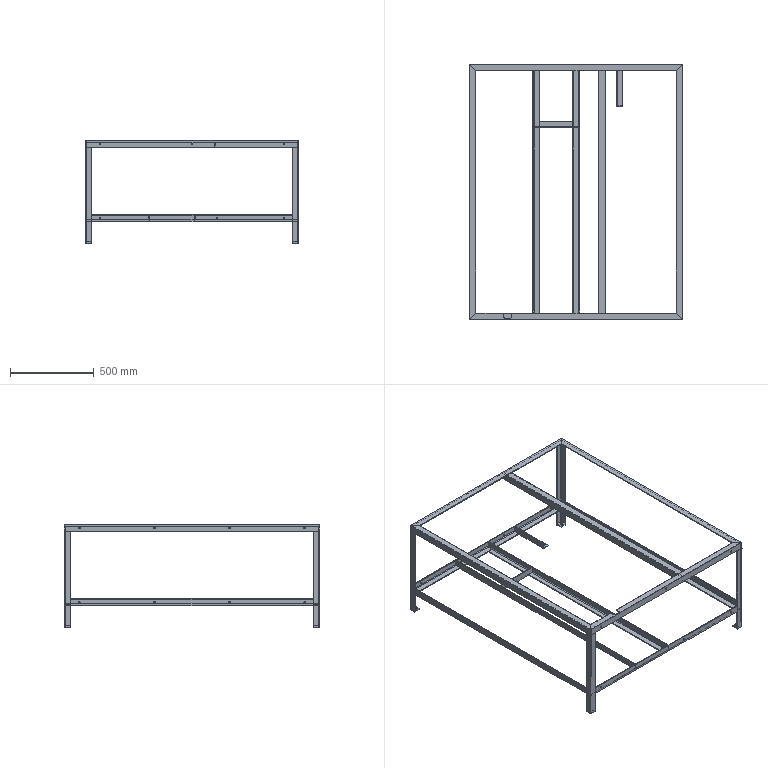Part | 21 solids | 354 faces | box 1280 x 1530 x 615 mm | volume 6883752 mm3 | plane 236 | cylinder 118 | commonest cylinder face diameters 10 x73 3.34 x35 14 x8 20 x2